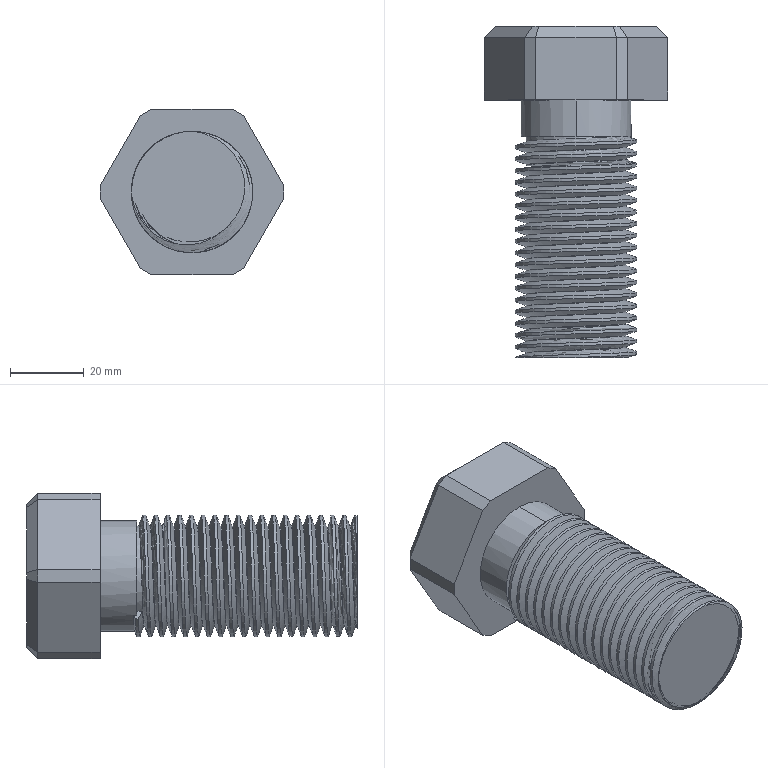Part | SolidWorks | features ICE 4, Chamfer 2, Extrusion 1, Helix 1, Sweep 1 | 1 solid | 73 faces | box 49.962 x 90 x 45 mm | volume 85439 mm3 | cylinder 41 | plane 29 | spline 3 | commonest cylinder face diameters 27 x39 30 x2